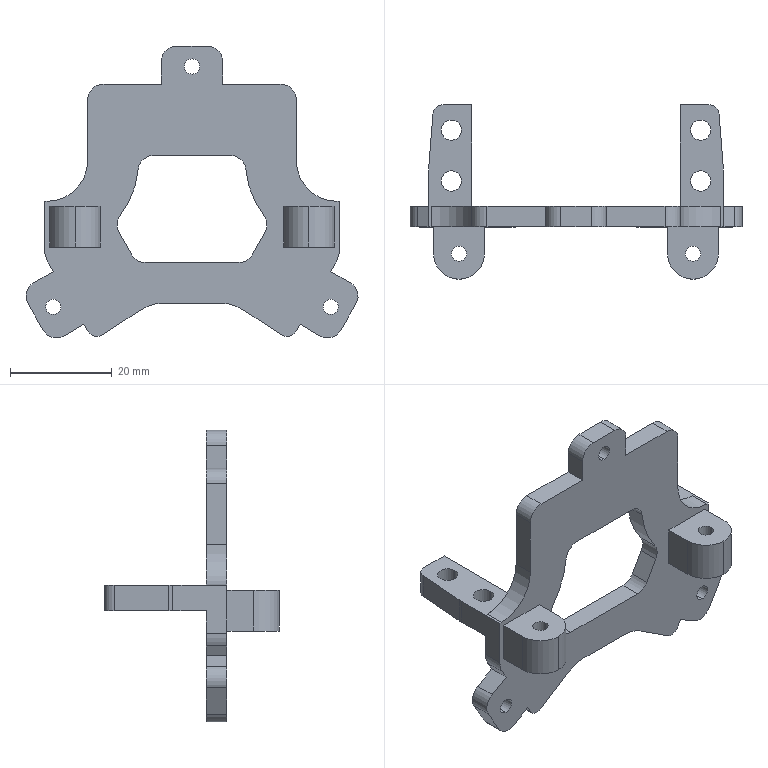Part | SolidWorks | features ICE 10, Fillet 6, HoleWzd 2, Extrusion 1, MirrorPattern 1 | 1 solid | 96 faces | box 65.292 x 34.3 x 57.348 mm | volume 10403 mm3 | cylinder 50 | plane 46 | commonest cylinder face diameters 6 x14 4 x12 3 x10 10 x6 16 x4 20 x2